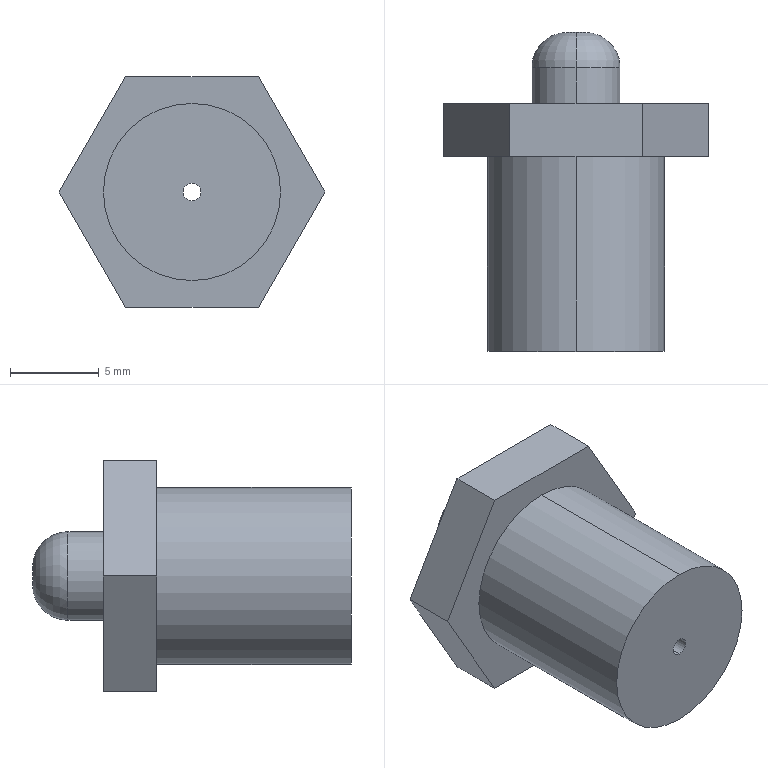Part | SolidWorks | features Fillet 1, ICE 1, Revolution 1 | 1 solid | 17 faces | box 15 x 18 x 12.99 mm | volume 1356 mm3 | plane 9 | cylinder 6 | torus 2 | commonest cylinder face diameters 1 x2 5 x2 10 x2
STEP:
#1=CARTESIAN_POINT('',(0.,18.,0.5));
#2=VERTEX_POINT('',#1);
#3=CARTESIAN_POINT('',(0.,18.,-0.5));
#4=VERTEX_POINT('',#3);
#5=CARTESIAN_POINT('',(0.,18.,0.));
#6=DIRECTION('',(0.,1.,0.));
#7=DIRECTION('',(0.,0.,1.));
#8=AXIS2_PLACEMENT_3D('',#5,#6,#7);
#9=CIRCLE('',#8,0.5);
#10=EDGE_CURVE('',#2,#4,#9,.T.);
#11=ORIENTED_EDGE('',*,*,#10,.F.);
#12=CARTESIAN_POINT('',(0.,16.,2.5));
#13=VERTEX_POINT('',#12);
#14=CARTESIAN_POINT('',(0.,16.,0.5));
#15=DIRECTION('',(1.,0.,0.));
#16=DIRECTION('',(0.,0.,-1.));
#17=AXIS2_PLACEMENT_3D('',#14,#15,#16);
#18=CIRCLE('',#17,2.);
#19=EDGE_CURVE('',#2,#13,#18,.T.);
#20=ORIENTED_EDGE('',*,*,#19,.T.);
#21=CARTESIAN_POINT('',(0.,16.,-2.5));
#22=VERTEX_POINT('',#21);
#23=CARTESIAN_POINT('',(0.,16.,0.));
#24=DIRECTION('',(0.,-1.,0.));
#25=DIRECTION('',(0.,0.,-1.));
#26=AXIS2_PLACEMENT_3D('',#23,#24,#25);
#27=CIRCLE('',#26,2.5);
#28=EDGE_CURVE('',#22,#13,#27,.T.);
#29=ORIENTED_EDGE('',*,*,#28,.F.);
#30=CARTESIAN_POINT('',(0.,16.,-0.5));
#31=DIRECTION('',(-1.,0.,0.));
#32=DIRECTION('',(0.,0.,1.));
#33=AXIS2_PLACEMENT_3D('',#30,#31,#32);
#34=CIRCLE('',#33,2.);
#35=EDGE_CURVE('',#4,#22,#34,.T.);
#36=ORIENTED_EDGE('',*,*,#35,.F.);
#37=EDGE_LOOP('',(#11,#20,#29,#36));
#38=FACE_OUTER_BOUND('',#37,.T.);
#39=CARTESIAN_POINT('',(0.,16.,0.));
#40=DIRECTION('',(0.,-1.,0.));
#41=DIRECTION('',(0.,0.,-1.));
#42=AXIS2_PLACEMENT_3D('',#39,#40,#41);
#43=TOROIDAL_SURFACE('',#42,0.5,2.);
#44=ADVANCED_FACE('',(#38),#43,.T.);
#45=CARTESIAN_POINT('',(0.,14.,2.5));
#46=VERTEX_POINT('',#45);
#47=CARTESIAN_POINT('',(0.,14.,-2.5));
#48=VERTEX_POINT('',#47);
#49=CARTESIAN_POINT('',(0.,14.,0.));
#50=DIRECTION('',(0.,1.,0.));
#51=DIRECTION('',(0.,0.,1.));
#52=AXIS2_PLACEMENT_3D('',#49,#50,#51);
#53=CIRCLE('',#52,2.5);
#54=EDGE_CURVE('',#46,#48,#53,.T.);
#55=ORIENTED_EDGE('',*,*,#54,.T.);
#56=CARTESIAN_POINT('',(0.,0.,-2.5));
#57=DIRECTION('',(0.,1.,0.));
#58=VECTOR('',#57,1000.);
#59=LINE('',#56,#58);
#60=EDGE_CURVE('',#48,#22,#59,.T.);
#61=ORIENTED_EDGE('',*,*,#60,.T.);
#62=ORIENTED_EDGE('',*,*,#28,.T.);
#63=CARTESIAN_POINT('',(0.,0.,2.5));
#64=DIRECTION('',(0.,1.,0.));
#65=VECTOR('',#64,1000.);
#66=LINE('',#63,#65);
#67=EDGE_CURVE('',#46,#13,#66,.T.);
#68=ORIENTED_EDGE('',*,*,#67,.F.);
#69=EDGE_LOOP('',(#55,#61,#62,#68));
#70=FACE_OUTER_BOUND('',#69,.T.);
#71=CARTESIAN_POINT('',(0.,0.,0.));
#72=DIRECTION('',(0.,1.,0.));
#73=DIRECTION('',(0.,0.,1.));
#74=AXIS2_PLACEMENT_3D('',#71,#72,#73);
#75=CYLINDRICAL_SURFACE('',#74,2.5);
#76=ADVANCED_FACE('',(#70),#75,.T.);
#77=CARTESIAN_POINT('',(0.,0.,-0.5));
#78=VERTEX_POINT('',#77);
#79=CARTESIAN_POINT('',(0.,0.,0.5));
#80=VERTEX_POINT('',#79);
#81=CARTESIAN_POINT('',(0.,0.,0.));
#82=DIRECTION('',(0.,1.,0.));
#83=DIRECTION('',(0.,0.,1.));
#84=AXIS2_PLACEMENT_3D('',#81,#82,#83);
#85=CIRCLE('',#84,0.5);
#86=EDGE_CURVE('',#78,#80,#85,.T.);
#87=ORIENTED_EDGE('',*,*,#86,.F.);
#88=CARTESIAN_POINT('',(0.,0.,-0.5));
#89=DIRECTION('',(0.,1.,0.));
#90=VECTOR('',#89,1000.);
#91=LINE('',#88,#90);
#92=EDGE_CURVE('',#78,#4,#91,.T.);
#93=ORIENTED_EDGE('',*,*,#92,.T.);
#94=CARTESIAN_POINT('',(0.,18.,0.));
#95=DIRECTION('',(0.,1.,0.));
#96=DIRECTION('',(0.,0.,1.));
#97=AXIS2_PLACEMENT_3D('',#94,#95,#96);
#98=CIRCLE('',#97,0.5);
#99=EDGE_CURVE('',#4,#2,#98,.T.);
#100=ORIENTED_EDGE('',*,*,#99,.T.);
#101=CARTESIAN_POINT('',(0.,0.,0.5));
#102=DIRECTION('',(0.,1.,0.));
#103=VECTOR('',#102,1000.);
#104=LINE('',#101,#103);
#105=EDGE_CURVE('',#80,#2,#104,.T.);
#106=ORIENTED_EDGE('',*,*,#105,.F.);
#107=EDGE_LOOP('',(#87,#93,#100,#106));
#108=FACE_OUTER_BOUND('',#107,.T.);
#109=CARTESIAN_POINT('',(0.,0.,0.));
#110=DIRECTION('',(0.,1.,0.));
#111=DIRECTION('',(0.,0.,1.));
#112=AXIS2_PLACEMENT_3D('',#109,#110,#111);
#113=CYLINDRICAL_SURFACE('',#112,0.5);
#114=ADVANCED_FACE('',(#108),#113,.F.);
#115=CARTESIAN_POINT('',(0.,0.,5.));
#116=VERTEX_POINT('',#115);
#117=CARTESIAN_POINT('',(0.,0.,-5.));
#118=VERTEX_POINT('',#117);
#119=CARTESIAN_POINT('',(0.,0.,0.));
#120=DIRECTION('',(0.,1.,0.));
#121=DIRECTION('',(0.,0.,1.));
#122=AXIS2_PLACEMENT_3D('',#119,#120,#121);
#123=CIRCLE('',#122,5.);
#124=EDGE_CURVE('',#116,#118,#123,.T.);
#125=ORIENTED_EDGE('',*,*,#124,.T.);
#126=CARTESIAN_POINT('',(0.,11.,-5.));
#127=VERTEX_POINT('',#126);
#128=CARTESIAN_POINT('',(0.,0.,-5.));
#129=DIRECTION('',(0.,1.,0.));
#130=VECTOR('',#129,1000.);
#131=LINE('',#128,#130);
#132=EDGE_CURVE('',#118,#127,#131,.T.);
#133=ORIENTED_EDGE('',*,*,#132,.T.);
#134=CARTESIAN_POINT('',(0.,11.,5.));
#135=VERTEX_POINT('',#134);
#136=CARTESIAN_POINT('',(0.,11.,0.));
#137=DIRECTION('',(0.,1.,0.));
#138=DIRECTION('',(0.,0.,1.));
#139=AXIS2_PLACEMENT_3D('',#136,#137,#138);
#140=CIRCLE('',#139,5.);
#141=EDGE_CURVE('',#135,#127,#140,.T.);
#142=ORIENTED_EDGE('',*,*,#141,.F.);
#143=CARTESIAN_POINT('',(0.,0.,5.));
#144=DIRECTION('',(0.,1.,0.));
#145=VECTOR('',#144,1000.);
#146=LINE('',#143,#145);
#147=EDGE_CURVE('',#116,#135,#146,.T.);
#148=ORIENTED_EDGE('',*,*,#147,.F.);
#149=EDGE_LOOP('',(#125,#133,#142,#148));
#150=FACE_OUTER_BOUND('',#149,.T.);
#151=CARTESIAN_POINT('',(0.,0.,0.));
#152=DIRECTION('',(0.,1.,0.));
#153=DIRECTION('',(0.,0.,1.));
#154=AXIS2_PLACEMENT_3D('',#151,#152,#153);
#155=CYLINDRICAL_SURFACE('',#154,5.);
#156=ADVANCED_FACE('',(#150),#155,.T.);
#157=ORIENTED_EDGE('',*,*,#54,.F.);
#158=CARTESIAN_POINT('',(0.,14.,0.));
#159=DIRECTION('',(0.,1.,0.));
#160=DIRECTION('',(0.,0.,1.));
#161=AXIS2_PLACEMENT_3D('',#158,#159,#160);
#162=CIRCLE('',#161,2.5);
#163=EDGE_CURVE('',#48,#46,#162,.T.);
#164=ORIENTED_EDGE('',*,*,#163,.F.);
#165=EDGE_LOOP('',(#157,#164));
#166=FACE_BOUND('',#165,.T.);
#167=CARTESIAN_POINT('',(-3.75,14.,-6.495));
#168=VERTEX_POINT('',#167);
#169=CARTESIAN_POINT('',(-7.5,14.,0.));
#170=VERTEX_POINT('',#169);
#171=CARTESIAN_POINT('',(-3.75,14.,-6.495));
#172=DIRECTION('',(-0.5,0.,0.866));
#173=VECTOR('',#172,1000.);
#174=LINE('',#171,#173);
#175=EDGE_CURVE('',#168,#170,#174,.T.);
#176=ORIENTED_EDGE('',*,*,#175,.T.);
#177=CARTESIAN_POINT('',(-3.75,14.,6.495));
#178=VERTEX_POINT('',#177);
#179=CARTESIAN_POINT('',(-7.5,14.,0.));
#180=DIRECTION('',(0.5,0.,0.866));
#181=VECTOR('',#180,1000.);
#182=LINE('',#179,#181);
#183=EDGE_CURVE('',#170,#178,#182,.T.);
#184=ORIENTED_EDGE('',*,*,#183,.T.);
#185=CARTESIAN_POINT('',(3.75,14.,6.495));
#186=VERTEX_POINT('',#185);
#187=CARTESIAN_POINT('',(-3.75,14.,6.495));
#188=DIRECTION('',(1.,0.,0.));
#189=VECTOR('',#188,1000.);
#190=LINE('',#187,#189);
#191=EDGE_CURVE('',#178,#186,#190,.T.);
#192=ORIENTED_EDGE('',*,*,#191,.T.);
#193=CARTESIAN_POINT('',(7.5,14.,0.));
#194=VERTEX_POINT('',#193);
#195=CARTESIAN_POINT('',(3.75,14.,6.495));
#196=DIRECTION('',(0.5,0.,-0.866));
#197=VECTOR('',#196,1000.);
#198=LINE('',#195,#197);
#199=EDGE_CURVE('',#186,#194,#198,.T.);
#200=ORIENTED_EDGE('',*,*,#199,.T.);
#201=CARTESIAN_POINT('',(3.75,14.,-6.495));
#202=VERTEX_POINT('',#201);
#203=CARTESIAN_POINT('',(7.5,14.,0.));
#204=DIRECTION('',(-0.5,0.,-0.866));
#205=VECTOR('',#204,1000.);
#206=LINE('',#203,#205);
#207=EDGE_CURVE('',#194,#202,#206,.T.);
#208=ORIENTED_EDGE('',*,*,#207,.T.);
#209=CARTESIAN_POINT('',(3.75,14.,-6.495));
#210=DIRECTION('',(-1.,0.,0.));
#211=VECTOR('',#210,1000.);
#212=LINE('',#209,#211);
#213=EDGE_CURVE('',#202,#168,#212,.T.);
#214=ORIENTED_EDGE('',*,*,#213,.T.);
#215=EDGE_LOOP('',(#176,#184,#192,#200,#208,#214));
#216=FACE_OUTER_BOUND('',#215,.T.);
#217=CARTESIAN_POINT('',(7.5,14.,0.));
#218=DIRECTION('',(0.,-1.,0.));
#219=DIRECTION('',(0.,0.,-1.));
#220=AXIS2_PLACEMENT_3D('',#217,#218,#219);
#221=PLANE('',#220);
#222=ADVANCED_FACE('',(#166,#216),#221,.F.);
#223=ORIENTED_EDGE('',*,*,#141,.T.);
#224=CARTESIAN_POINT('',(0.,11.,0.));
#225=DIRECTION('',(0.,1.,0.));
#226=DIRECTION('',(0.,0.,1.));
#227=AXIS2_PLACEMENT_3D('',#224,#225,#226);
#228=CIRCLE('',#227,5.);
#229=EDGE_CURVE('',#127,#135,#228,.T.);
#230=ORIENTED_EDGE('',*,*,#229,.T.);
#231=EDGE_LOOP('',(#223,#230));
#232=FACE_BOUND('',#231,.T.);
#233=CARTESIAN_POINT('',(-3.75,11.,-6.495));
#234=VERTEX_POINT('',#233);
#235=CARTESIAN_POINT('',(-7.5,11.,0.));
#236=VERTEX_POINT('',#235);
#237=CARTESIAN_POINT('',(-4.375,11.,-5.413));
#238=DIRECTION('',(-0.5,0.,0.866));
#239=VECTOR('',#238,1000.);
#240=LINE('',#237,#239);
#241=EDGE_CURVE('',#234,#236,#240,.T.);
#242=ORIENTED_EDGE('',*,*,#241,.F.);
#243=CARTESIAN_POINT('',(3.75,11.,-6.495));
#244=VERTEX_POINT('',#243);
#245=CARTESIAN_POINT('',(5.,11.,-6.495));
#246=DIRECTION('',(-1.,0.,0.));
#247=VECTOR('',#246,1000.);
#248=LINE('',#245,#247);
#249=EDGE_CURVE('',#244,#234,#248,.T.);
#250=ORIENTED_EDGE('',*,*,#249,.F.);
#251=CARTESIAN_POINT('',(7.5,11.,0.));
#252=VERTEX_POINT('',#251);
#253=CARTESIAN_POINT('',(6.875,11.,-1.083));
#254=DIRECTION('',(-0.5,0.,-0.866));
#255=VECTOR('',#254,1000.);
#256=LINE('',#253,#255);
#257=EDGE_CURVE('',#252,#244,#256,.T.);
#258=ORIENTED_EDGE('',*,*,#257,.F.);
#259=CARTESIAN_POINT('',(3.75,11.,6.495));
#260=VERTEX_POINT('',#259);
#261=CARTESIAN_POINT('',(6.875,11.,1.083));
#262=DIRECTION('',(0.5,0.,-0.866));
#263=VECTOR('',#262,1000.);
#264=LINE('',#261,#263);
#265=EDGE_CURVE('',#260,#252,#264,.T.);
#266=ORIENTED_EDGE('',*,*,#265,.F.);
#267=CARTESIAN_POINT('',(-3.75,11.,6.495));
#268=VERTEX_POINT('',#267);
#269=CARTESIAN_POINT('',(5.,11.,6.495));
#270=DIRECTION('',(1.,0.,0.));
#271=VECTOR('',#270,1000.);
#272=LINE('',#269,#271);
#273=EDGE_CURVE('',#268,#260,#272,.T.);
#274=ORIENTED_EDGE('',*,*,#273,.F.);
#275=CARTESIAN_POINT('',(-4.375,11.,5.413));
#276=DIRECTION('',(0.5,0.,0.866));
#277=VECTOR('',#276,1000.);
#278=LINE('',#275,#277);
#279=EDGE_CURVE('',#236,#268,#278,.T.);
#280=ORIENTED_EDGE('',*,*,#279,.F.);
#281=EDGE_LOOP('',(#242,#250,#258,#266,#274,#280));
#282=FACE_OUTER_BOUND('',#281,.T.);
#283=CARTESIAN_POINT('',(5.,11.,0.));
#284=DIRECTION('',(0.,1.,0.));
#285=DIRECTION('',(0.,0.,1.));
#286=AXIS2_PLACEMENT_3D('',#283,#284,#285);
#287=PLANE('',#286);
#288=ADVANCED_FACE('',(#232,#282),#287,.F.);
#289=ORIENTED_EDGE('',*,*,#132,.F.);
#290=CARTESIAN_POINT('',(0.,0.,0.));
#291=DIRECTION('',(0.,1.,0.));
#292=DIRECTION('',(0.,0.,1.));
#293=AXIS2_PLACEMENT_3D('',#290,#291,#292);
#294=CIRCLE('',#293,5.);
#295=EDGE_CURVE('',#118,#116,#294,.T.);
#296=ORIENTED_EDGE('',*,*,#295,.T.);
#297=ORIENTED_EDGE('',*,*,#147,.T.);
#298=ORIENTED_EDGE('',*,*,#229,.F.);
#299=EDGE_LOOP('',(#289,#296,#297,#298));
#300=FACE_OUTER_BOUND('',#299,.T.);
#301=CARTESIAN_POINT('',(0.,0.,0.));
#302=DIRECTION('',(0.,1.,0.));
#303=DIRECTION('',(0.,0.,1.));
#304=AXIS2_PLACEMENT_3D('',#301,#302,#303);
#305=CYLINDRICAL_SURFACE('',#304,5.);
#306=ADVANCED_FACE('',(#300),#305,.T.);
#307=ORIENTED_EDGE('',*,*,#124,.F.);
#308=ORIENTED_EDGE('',*,*,#295,.F.);
#309=EDGE_LOOP('',(#307,#308));
#310=FACE_OUTER_BOUND('',#309,.T.);
#311=CARTESIAN_POINT('',(0.,0.,0.));
#312=DIRECTION('',(0.,1.,0.));
#313=DIRECTION('',(0.,0.,1.));
#314=AXIS2_PLACEMENT_3D('',#311,#312,#313);
#315=CIRCLE('',#314,0.5);
#316=EDGE_CURVE('',#80,#78,#315,.T.);
#317=ORIENTED_EDGE('',*,*,#316,.T.);
#318=ORIENTED_EDGE('',*,*,#86,.T.);
#319=EDGE_LOOP('',(#317,#318));
#320=FACE_BOUND('',#319,.T.);
#321=CARTESIAN_POINT('',(0.5,0.,0.));
#322=DIRECTION('',(0.,1.,0.));
#323=DIRECTION('',(0.,0.,1.));
#324=AXIS2_PLACEMENT_3D('',#321,#322,#323);
#325=PLANE('',#324);
#326=ADVANCED_FACE('',(#310,#320),#325,.F.);
#327=ORIENTED_EDGE('',*,*,#92,.F.);
#328=ORIENTED_EDGE('',*,*,#316,.F.);
#329=ORIENTED_EDGE('',*,*,#105,.T.);
#330=ORIENTED_EDGE('',*,*,#10,.T.);
#331=EDGE_LOOP('',(#327,#328,#329,#330));
#332=FACE_OUTER_BOUND('',#331,.T.);
#333=CARTESIAN_POINT('',(0.,0.,0.));
#334=DIRECTION('',(0.,1.,0.));
#335=DIRECTION('',(0.,0.,1.));
#336=AXIS2_PLACEMENT_3D('',#333,#334,#335);
#337=CYLINDRICAL_SURFACE('',#336,0.5);
#338=ADVANCED_FACE('',(#332),#337,.F.);
#339=ORIENTED_EDGE('',*,*,#60,.F.);
#340=ORIENTED_EDGE('',*,*,#163,.T.);
#341=ORIENTED_EDGE('',*,*,#67,.T.);
#342=CARTESIAN_POINT('',(0.,16.,0.));
#343=DIRECTION('',(0.,-1.,0.));
#344=DIRECTION('',(0.,0.,-1.));
#345=AXIS2_PLACEMENT_3D('',#342,#343,#344);
#346=CIRCLE('',#345,2.5);
#347=EDGE_CURVE('',#13,#22,#346,.T.);
#348=ORIENTED_EDGE('',*,*,#347,.T.);
#349=EDGE_LOOP('',(#339,#340,#341,#348));
#350=FACE_OUTER_BOUND('',#349,.T.);
#351=CARTESIAN_POINT('',(0.,0.,0.));
#352=DIRECTION('',(0.,1.,0.));
#353=DIRECTION('',(0.,0.,1.));
#354=AXIS2_PLACEMENT_3D('',#351,#352,#353);
#355=CYLINDRICAL_SURFACE('',#354,2.5);
#356=ADVANCED_FACE('',(#350),#355,.T.);
#357=ORIENTED_EDGE('',*,*,#241,.T.);
#358=CARTESIAN_POINT('',(-7.5,4.,0.));
#359=DIRECTION('',(0.,1.,0.));
#360=VECTOR('',#359,1000.);
#361=LINE('',#358,#360);
#362=EDGE_CURVE('',#236,#170,#361,.T.);
#363=ORIENTED_EDGE('',*,*,#362,.T.);
#364=ORIENTED_EDGE('',*,*,#175,.F.);
#365=CARTESIAN_POINT('',(-3.75,4.,-6.495));
#366=DIRECTION('',(0.,1.,0.));
#367=VECTOR('',#366,1000.);
#368=LINE('',#365,#367);
#369=EDGE_CURVE('',#234,#168,#368,.T.);
#370=ORIENTED_EDGE('',*,*,#369,.F.);
#371=EDGE_LOOP('',(#357,#363,#364,#370));
#372=FACE_OUTER_BOUND('',#371,.T.);
#373=CARTESIAN_POINT('',(-3.75,4.,-6.495));
#374=DIRECTION('',(-0.866,0.,-0.5));
#375=DIRECTION('',(-0.5,0.,0.866));
#376=AXIS2_PLACEMENT_3D('',#373,#374,#375);
#377=PLANE('',#376);
#378=ADVANCED_FACE('',(#372),#377,.T.);
#379=ORIENTED_EDGE('',*,*,#249,.T.);
#380=ORIENTED_EDGE('',*,*,#369,.T.);
#381=ORIENTED_EDGE('',*,*,#213,.F.);
#382=CARTESIAN_POINT('',(3.75,4.,-6.495));
#383=DIRECTION('',(0.,1.,0.));
#384=VECTOR('',#383,1000.);
#385=LINE('',#382,#384);
#386=EDGE_CURVE('',#244,#202,#385,.T.);
#387=ORIENTED_EDGE('',*,*,#386,.F.);
#388=EDGE_LOOP('',(#379,#380,#381,#387));
#389=FACE_OUTER_BOUND('',#388,.T.);
#390=CARTESIAN_POINT('',(3.75,4.,-6.495));
#391=DIRECTION('',(0.,0.,-1.));
#392=DIRECTION('',(-1.,0.,0.));
#393=AXIS2_PLACEMENT_3D('',#390,#391,#392);
#394=PLANE('',#393);
#395=ADVANCED_FACE('',(#389),#394,.T.);
#396=ORIENTED_EDGE('',*,*,#257,.T.);
#397=ORIENTED_EDGE('',*,*,#386,.T.);
#398=ORIENTED_EDGE('',*,*,#207,.F.);
#399=CARTESIAN_POINT('',(7.5,4.,0.));
#400=DIRECTION('',(0.,1.,0.));
#401=VECTOR('',#400,1000.);
#402=LINE('',#399,#401);
#403=EDGE_CURVE('',#252,#194,#402,.T.);
#404=ORIENTED_EDGE('',*,*,#403,.F.);
#405=EDGE_LOOP('',(#396,#397,#398,#404));
#406=FACE_OUTER_BOUND('',#405,.T.);
#407=CARTESIAN_POINT('',(7.5,4.,0.));
#408=DIRECTION('',(0.866,0.,-0.5));
#409=DIRECTION('',(-0.5,0.,-0.866));
#410=AXIS2_PLACEMENT_3D('',#407,#408,#409);
#411=PLANE('',#410);
#412=ADVANCED_FACE('',(#406),#411,.T.);
#413=ORIENTED_EDGE('',*,*,#265,.T.);
#414=ORIENTED_EDGE('',*,*,#403,.T.);
#415=ORIENTED_EDGE('',*,*,#199,.F.);
#416=CARTESIAN_POINT('',(3.75,4.,6.495));
#417=DIRECTION('',(0.,1.,0.));
#418=VECTOR('',#417,1000.);
#419=LINE('',#416,#418);
#420=EDGE_CURVE('',#260,#186,#419,.T.);
#421=ORIENTED_EDGE('',*,*,#420,.F.);
#422=EDGE_LOOP('',(#413,#414,#415,#421));
#423=FACE_OUTER_BOUND('',#422,.T.);
#424=CARTESIAN_POINT('',(3.75,4.,6.495));
#425=DIRECTION('',(0.866,0.,0.5));
#426=DIRECTION('',(0.5,0.,-0.866));
#427=AXIS2_PLACEMENT_3D('',#424,#425,#426);
#428=PLANE('',#427);
#429=ADVANCED_FACE('',(#423),#428,.T.);
#430=ORIENTED_EDGE('',*,*,#273,.T.);
#431=ORIENTED_EDGE('',*,*,#420,.T.);
#432=ORIENTED_EDGE('',*,*,#191,.F.);
#433=CARTESIAN_POINT('',(-3.75,4.,6.495));
#434=DIRECTION('',(0.,1.,0.));
#435=VECTOR('',#434,1000.);
#436=LINE('',#433,#435);
#437=EDGE_CURVE('',#268,#178,#436,.T.);
#438=ORIENTED_EDGE('',*,*,#437,.F.);
#439=EDGE_LOOP('',(#430,#431,#432,#438));
#440=FACE_OUTER_BOUND('',#439,.T.);
#441=CARTESIAN_POINT('',(-3.75,4.,6.495));
#442=DIRECTION('',(0.,0.,1.));
#443=DIRECTION('',(1.,0.,0.));
#444=AXIS2_PLACEMENT_3D('',#441,#442,#443);
#445=PLANE('',#444);
#446=ADVANCED_FACE('',(#440),#445,.T.);
#447=ORIENTED_EDGE('',*,*,#279,.T.);
#448=ORIENTED_EDGE('',*,*,#437,.T.);
#449=ORIENTED_EDGE('',*,*,#183,.F.);
#450=ORIENTED_EDGE('',*,*,#362,.F.);
#451=EDGE_LOOP('',(#447,#448,#449,#450));
#452=FACE_OUTER_BOUND('',#451,.T.);
#453=CARTESIAN_POINT('',(-7.5,4.,0.));
#454=DIRECTION('',(-0.866,0.,0.5));
#455=DIRECTION('',(0.5,0.,0.866));
#456=AXIS2_PLACEMENT_3D('',#453,#454,#455);
#457=PLANE('',#456);
#458=ADVANCED_FACE('',(#452),#457,.T.);
#459=ORIENTED_EDGE('',*,*,#19,.F.);
#460=ORIENTED_EDGE('',*,*,#99,.F.);
#461=ORIENTED_EDGE('',*,*,#35,.T.);
#462=ORIENTED_EDGE('',*,*,#347,.F.);
#463=EDGE_LOOP('',(#459,#460,#461,#462));
#464=FACE_OUTER_BOUND('',#463,.T.);
#465=CARTESIAN_POINT('',(0.,16.,0.));
#466=DIRECTION('',(0.,-1.,0.));
#467=DIRECTION('',(0.,0.,-1.));
#468=AXIS2_PLACEMENT_3D('',#465,#466,#467);
#469=TOROIDAL_SURFACE('',#468,0.5,2.);
#470=ADVANCED_FACE('',(#464),#469,.T.);
#471=CLOSED_SHELL('',(#44,#76,#114,#156,#222,#288,#306,#326,#338,#356,#378,#395,#412,#429,#446,#458,#470));
#472=MANIFOLD_SOLID_BREP('',#471);
#473=CARTESIAN_POINT('',(0.,0.,0.));
#474=DIRECTION('',(0.,0.,1.));
#475=DIRECTION('',(1.,0.,0.));
#476=AXIS2_PLACEMENT_3D('',#473,#474,#475);
#477=(LENGTH_UNIT()NAMED_UNIT(*)SI_UNIT(.MILLI.,.METRE.));
#478=UNCERTAINTY_MEASURE_WITH_UNIT(LENGTH_MEASURE(0.00001),#477,'','');
#479=(NAMED_UNIT(*)PLANE_ANGLE_UNIT()SI_UNIT($,.RADIAN.));
#480=(NAMED_UNIT(*)SI_UNIT($,.STERADIAN.)SOLID_ANGLE_UNIT());
#481=(GEOMETRIC_REPRESENTATION_CONTEXT(3)GLOBAL_UNCERTAINTY_ASSIGNED_CONTEXT((#478))GLOBAL_UNIT_ASSIGNED_CONTEXT((#477,#479,#480))REPRESENTATION_CONTEXT('',''));
#482=ADVANCED_BREP_SHAPE_REPRESENTATION('',(#472,#476),#481);